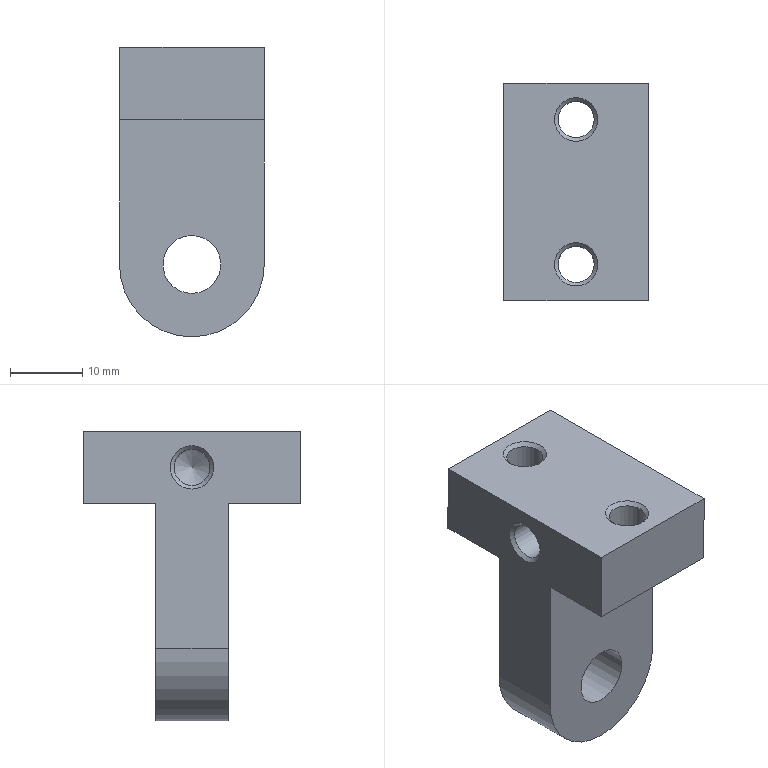Part | STEP file | 冲床-300配套压波_id686_x_t | 1 solid | 20 faces | box 20.046 x 30 x 40.015 mm | volume 10464 mm3 | plane 9 | cone 6 | cylinder 5 | commonest cylinder face diameters 5 x3 8 x1 20 x1
STEP:
#1=CARTESIAN_POINT('',(2189.7,-5.,-434.542));
#2=VERTEX_POINT('',#1);
#3=CARTESIAN_POINT('',(2193.457,-5.,-435.916));
#4=DIRECTION('',(0.,-1.,0.));
#5=DIRECTION('',(-0.9392,0.,0.3435));
#6=AXIS2_PLACEMENT_3D('',#3,#4,#5);
#7=CIRCLE('',#6,4.);
#8=EDGE_CURVE('',#2,#2,#7,.T.);
#9=ORIENTED_EDGE('',*,*,#8,.F.);
#10=EDGE_LOOP('',(#9));
#11=FACE_BOUND('',#10,.T.);
#12=CARTESIAN_POINT('',(2183.488,-5.,-415.901));
#13=VERTEX_POINT('',#12);
#14=CARTESIAN_POINT('',(2203.488,-5.,-415.931));
#15=VERTEX_POINT('',#14);
#16=CARTESIAN_POINT('',(2183.488,-5.,-415.901));
#17=DIRECTION('',(1.,0.,-0.001532));
#18=VECTOR('',#17,1.);
#19=LINE('',#16,#18);
#20=EDGE_CURVE('',#13,#15,#19,.T.);
#21=ORIENTED_EDGE('',*,*,#20,.F.);
#22=CARTESIAN_POINT('',(2183.457,-5.,-435.901));
#23=VERTEX_POINT('',#22);
#24=CARTESIAN_POINT('',(2183.48,-5.,-420.901));
#25=DIRECTION('',(-0.001532,0.,-1.));
#26=VECTOR('',#25,1.);
#27=LINE('',#24,#26);
#28=EDGE_CURVE('',#13,#23,#27,.T.);
#29=ORIENTED_EDGE('',*,*,#28,.T.);
#30=CARTESIAN_POINT('',(2203.457,-5.,-435.931));
#31=VERTEX_POINT('',#30);
#32=CARTESIAN_POINT('',(2193.457,-5.,-435.916));
#33=DIRECTION('',(0.,-1.,0.));
#34=DIRECTION('',(-1.,0.,0.001532));
#35=AXIS2_PLACEMENT_3D('',#32,#33,#34);
#36=CIRCLE('',#35,10.);
#37=EDGE_CURVE('',#23,#31,#36,.T.);
#38=ORIENTED_EDGE('',*,*,#37,.T.);
#39=CARTESIAN_POINT('',(2203.48,-5.,-420.931));
#40=DIRECTION('',(0.001532,0.,1.));
#41=VECTOR('',#40,1.);
#42=LINE('',#39,#41);
#43=EDGE_CURVE('',#31,#15,#42,.T.);
#44=ORIENTED_EDGE('',*,*,#43,.T.);
#45=EDGE_LOOP('',(#21,#29,#38,#44));
#46=FACE_BOUND('',#45,.T.);
#47=CARTESIAN_POINT('',(2183.48,-5.,-420.901));
#48=DIRECTION('',(0.,1.,0.));
#49=DIRECTION('',(1.,0.,-0.001532));
#50=AXIS2_PLACEMENT_3D('',#47,#48,#49);
#51=PLANE('',#50);
#52=ADVANCED_FACE('',(#11,#46),#51,.F.);
#53=CARTESIAN_POINT('',(2203.503,15.,-405.931));
#54=VERTEX_POINT('',#53);
#55=CARTESIAN_POINT('',(2203.503,-15.,-405.931));
#56=VERTEX_POINT('',#55);
#57=CARTESIAN_POINT('',(2203.503,5.,-405.931));
#58=DIRECTION('',(0.,-1.,0.));
#59=VECTOR('',#58,1.);
#60=LINE('',#57,#59);
#61=EDGE_CURVE('',#54,#56,#60,.T.);
#62=ORIENTED_EDGE('',*,*,#61,.T.);
#63=CARTESIAN_POINT('',(2203.488,-15.,-415.931));
#64=VERTEX_POINT('',#63);
#65=CARTESIAN_POINT('',(2203.495,-15.,-410.931));
#66=DIRECTION('',(0.001532,0.,1.));
#67=VECTOR('',#66,1.);
#68=LINE('',#65,#67);
#69=EDGE_CURVE('',#64,#56,#68,.T.);
#70=ORIENTED_EDGE('',*,*,#69,.F.);
#71=CARTESIAN_POINT('',(2203.488,5.,-415.931));
#72=DIRECTION('',(0.,-1.,0.));
#73=VECTOR('',#72,1.);
#74=LINE('',#71,#73);
#75=EDGE_CURVE('',#15,#64,#74,.T.);
#76=ORIENTED_EDGE('',*,*,#75,.F.);
#77=ORIENTED_EDGE('',*,*,#43,.F.);
#78=CARTESIAN_POINT('',(2203.457,5.,-435.931));
#79=VERTEX_POINT('',#78);
#80=CARTESIAN_POINT('',(2203.457,-48.5,-435.931));
#81=DIRECTION('',(0.,1.,0.));
#82=VECTOR('',#81,1.);
#83=LINE('',#80,#82);
#84=EDGE_CURVE('',#31,#79,#83,.T.);
#85=ORIENTED_EDGE('',*,*,#84,.T.);
#86=CARTESIAN_POINT('',(2203.488,5.,-415.931));
#87=VERTEX_POINT('',#86);
#88=CARTESIAN_POINT('',(2203.48,5.,-420.931));
#89=DIRECTION('',(-0.001532,0.,-1.));
#90=VECTOR('',#89,1.);
#91=LINE('',#88,#90);
#92=EDGE_CURVE('',#87,#79,#91,.T.);
#93=ORIENTED_EDGE('',*,*,#92,.F.);
#94=CARTESIAN_POINT('',(2203.488,15.,-415.931));
#95=VERTEX_POINT('',#94);
#96=CARTESIAN_POINT('',(2203.488,-5.,-415.931));
#97=DIRECTION('',(0.,-1.,0.));
#98=VECTOR('',#97,1.);
#99=LINE('',#96,#98);
#100=EDGE_CURVE('',#95,#87,#99,.T.);
#101=ORIENTED_EDGE('',*,*,#100,.F.);
#102=CARTESIAN_POINT('',(2203.495,15.,-410.931));
#103=DIRECTION('',(-0.001532,0.,-1.));
#104=VECTOR('',#103,1.);
#105=LINE('',#102,#104);
#106=EDGE_CURVE('',#54,#95,#105,.T.);
#107=ORIENTED_EDGE('',*,*,#106,.F.);
#108=EDGE_LOOP('',(#62,#70,#76,#77,#85,#93,#101,#107));
#109=FACE_OUTER_BOUND('',#108,.T.);
#110=CARTESIAN_POINT('',(2203.48,5.,-420.931));
#111=DIRECTION('',(1.,0.,-0.001532));
#112=DIRECTION('',(0.,1.,0.));
#113=AXIS2_PLACEMENT_3D('',#110,#111,#112);
#114=PLANE('',#113);
#115=ADVANCED_FACE('',(#109),#114,.T.);
#116=ORIENTED_EDGE('',*,*,#106,.T.);
#117=CARTESIAN_POINT('',(2183.488,15.,-415.901));
#118=VERTEX_POINT('',#117);
#119=CARTESIAN_POINT('',(2183.488,15.,-415.901));
#120=DIRECTION('',(-1.,0.,0.001532));
#121=VECTOR('',#120,1.);
#122=LINE('',#119,#121);
#123=EDGE_CURVE('',#95,#118,#122,.T.);
#124=ORIENTED_EDGE('',*,*,#123,.T.);
#125=CARTESIAN_POINT('',(2183.503,15.,-405.901));
#126=VERTEX_POINT('',#125);
#127=CARTESIAN_POINT('',(2183.495,15.,-410.901));
#128=DIRECTION('',(-0.001532,0.,-1.));
#129=VECTOR('',#128,1.);
#130=LINE('',#127,#129);
#131=EDGE_CURVE('',#126,#118,#130,.T.);
#132=ORIENTED_EDGE('',*,*,#131,.F.);
#133=CARTESIAN_POINT('',(2183.503,15.,-405.901));
#134=DIRECTION('',(-1.,0.,0.001532));
#135=VECTOR('',#134,1.);
#136=LINE('',#133,#135);
#137=EDGE_CURVE('',#54,#126,#136,.T.);
#138=ORIENTED_EDGE('',*,*,#137,.F.);
#139=EDGE_LOOP('',(#116,#124,#132,#138));
#140=FACE_OUTER_BOUND('',#139,.T.);
#141=CARTESIAN_POINT('',(2183.495,15.,-410.901));
#142=DIRECTION('',(0.,-1.,0.));
#143=DIRECTION('',(1.,0.,-0.001532));
#144=AXIS2_PLACEMENT_3D('',#141,#142,#143);
#145=PLANE('',#144);
#146=ADVANCED_FACE('',(#140),#145,.F.);
#147=CARTESIAN_POINT('',(2183.491,0.,-413.901));
#148=VERTEX_POINT('',#147);
#149=CARTESIAN_POINT('',(2183.495,0.,-410.901));
#150=DIRECTION('',(1.,0.,-0.001532));
#151=DIRECTION('',(-0.001532,0.,-1.));
#152=AXIS2_PLACEMENT_3D('',#149,#150,#151);
#153=CIRCLE('',#152,3.);
#154=EDGE_CURVE('',#148,#148,#153,.T.);
#155=ORIENTED_EDGE('',*,*,#154,.T.);
#156=EDGE_LOOP('',(#155));
#157=FACE_BOUND('',#156,.T.);
#158=CARTESIAN_POINT('',(2183.488,5.,-415.901));
#159=VERTEX_POINT('',#158);
#160=CARTESIAN_POINT('',(2183.488,5.,-415.901));
#161=DIRECTION('',(0.,-1.,0.));
#162=VECTOR('',#161,1.);
#163=LINE('',#160,#162);
#164=EDGE_CURVE('',#118,#159,#163,.T.);
#165=ORIENTED_EDGE('',*,*,#164,.T.);
#166=CARTESIAN_POINT('',(2183.457,5.,-435.901));
#167=VERTEX_POINT('',#166);
#168=CARTESIAN_POINT('',(2183.457,5.,-435.901));
#169=DIRECTION('',(0.001532,0.,1.));
#170=VECTOR('',#169,1.);
#171=LINE('',#168,#170);
#172=EDGE_CURVE('',#167,#159,#171,.T.);
#173=ORIENTED_EDGE('',*,*,#172,.F.);
#174=CARTESIAN_POINT('',(2183.457,-48.5,-435.901));
#175=DIRECTION('',(0.,1.,0.));
#176=VECTOR('',#175,1.);
#177=LINE('',#174,#176);
#178=EDGE_CURVE('',#23,#167,#177,.T.);
#179=ORIENTED_EDGE('',*,*,#178,.F.);
#180=ORIENTED_EDGE('',*,*,#28,.F.);
#181=CARTESIAN_POINT('',(2183.488,-15.,-415.901));
#182=VERTEX_POINT('',#181);
#183=CARTESIAN_POINT('',(2183.488,-5.,-415.901));
#184=DIRECTION('',(0.,-1.,0.));
#185=VECTOR('',#184,1.);
#186=LINE('',#183,#185);
#187=EDGE_CURVE('',#13,#182,#186,.T.);
#188=ORIENTED_EDGE('',*,*,#187,.T.);
#189=CARTESIAN_POINT('',(2183.503,-15.,-405.901));
#190=VERTEX_POINT('',#189);
#191=CARTESIAN_POINT('',(2183.495,-15.,-410.901));
#192=DIRECTION('',(0.001532,0.,1.));
#193=VECTOR('',#192,1.);
#194=LINE('',#191,#193);
#195=EDGE_CURVE('',#182,#190,#194,.T.);
#196=ORIENTED_EDGE('',*,*,#195,.T.);
#197=CARTESIAN_POINT('',(2183.503,5.,-405.901));
#198=DIRECTION('',(0.,-1.,0.));
#199=VECTOR('',#198,1.);
#200=LINE('',#197,#199);
#201=EDGE_CURVE('',#126,#190,#200,.T.);
#202=ORIENTED_EDGE('',*,*,#201,.F.);
#203=ORIENTED_EDGE('',*,*,#131,.T.);
#204=EDGE_LOOP('',(#165,#173,#179,#180,#188,#196,#202,#203));
#205=FACE_BOUND('',#204,.T.);
#206=CARTESIAN_POINT('',(2183.48,5.,-420.901));
#207=DIRECTION('',(1.,0.,-0.001532));
#208=DIRECTION('',(0.,1.,0.));
#209=AXIS2_PLACEMENT_3D('',#206,#207,#208);
#210=PLANE('',#209);
#211=ADVANCED_FACE('',(#157,#205),#210,.F.);
#212=CARTESIAN_POINT('',(2190.503,10.,-405.911));
#213=VERTEX_POINT('',#212);
#214=CARTESIAN_POINT('',(2193.503,10.,-405.916));
#215=DIRECTION('',(-0.001532,0.,-1.));
#216=DIRECTION('',(-1.,0.,0.001532));
#217=AXIS2_PLACEMENT_3D('',#214,#215,#216);
#218=CIRCLE('',#217,3.);
#219=EDGE_CURVE('',#213,#213,#218,.T.);
#220=ORIENTED_EDGE('',*,*,#219,.T.);
#221=EDGE_LOOP('',(#220));
#222=FACE_BOUND('',#221,.T.);
#223=CARTESIAN_POINT('',(2190.503,-10.,-405.911));
#224=VERTEX_POINT('',#223);
#225=CARTESIAN_POINT('',(2193.503,-10.,-405.916));
#226=DIRECTION('',(-0.001532,0.,-1.));
#227=DIRECTION('',(-1.,0.,0.001532));
#228=AXIS2_PLACEMENT_3D('',#225,#226,#227);
#229=CIRCLE('',#228,3.);
#230=EDGE_CURVE('',#224,#224,#229,.T.);
#231=ORIENTED_EDGE('',*,*,#230,.T.);
#232=EDGE_LOOP('',(#231));
#233=FACE_BOUND('',#232,.T.);
#234=ORIENTED_EDGE('',*,*,#137,.T.);
#235=ORIENTED_EDGE('',*,*,#201,.T.);
#236=CARTESIAN_POINT('',(2183.503,-15.,-405.901));
#237=DIRECTION('',(1.,0.,-0.001532));
#238=VECTOR('',#237,1.);
#239=LINE('',#236,#238);
#240=EDGE_CURVE('',#190,#56,#239,.T.);
#241=ORIENTED_EDGE('',*,*,#240,.T.);
#242=ORIENTED_EDGE('',*,*,#61,.F.);
#243=EDGE_LOOP('',(#234,#235,#241,#242));
#244=FACE_BOUND('',#243,.T.);
#245=CARTESIAN_POINT('',(2183.503,5.,-405.901));
#246=DIRECTION('',(-0.001532,0.,-1.));
#247=DIRECTION('',(-1.,0.,0.001532));
#248=AXIS2_PLACEMENT_3D('',#245,#246,#247);
#249=PLANE('',#248);
#250=ADVANCED_FACE('',(#222,#233,#244),#249,.F.);
#251=CARTESIAN_POINT('',(2190.488,10.,-415.911));
#252=VERTEX_POINT('',#251);
#253=CARTESIAN_POINT('',(2193.488,10.,-415.916));
#254=DIRECTION('',(0.001532,0.,1.));
#255=DIRECTION('',(-1.,0.,0.001532));
#256=AXIS2_PLACEMENT_3D('',#253,#254,#255);
#257=CIRCLE('',#256,3.);
#258=EDGE_CURVE('',#252,#252,#257,.T.);
#259=ORIENTED_EDGE('',*,*,#258,.T.);
#260=EDGE_LOOP('',(#259));
#261=FACE_BOUND('',#260,.T.);
#262=CARTESIAN_POINT('',(2163.488,5.,-415.87));
#263=DIRECTION('',(1.,0.,-0.001532));
#264=VECTOR('',#263,1.);
#265=LINE('',#262,#264);
#266=EDGE_CURVE('',#159,#87,#265,.T.);
#267=ORIENTED_EDGE('',*,*,#266,.F.);
#268=ORIENTED_EDGE('',*,*,#164,.F.);
#269=ORIENTED_EDGE('',*,*,#123,.F.);
#270=ORIENTED_EDGE('',*,*,#100,.T.);
#271=EDGE_LOOP('',(#267,#268,#269,#270));
#272=FACE_BOUND('',#271,.T.);
#273=CARTESIAN_POINT('',(2183.488,-5.,-415.901));
#274=DIRECTION('',(-0.001532,0.,-1.));
#275=DIRECTION('',(-1.,0.,0.001532));
#276=AXIS2_PLACEMENT_3D('',#273,#274,#275);
#277=PLANE('',#276);
#278=ADVANCED_FACE('',(#261,#272),#277,.T.);
#279=CARTESIAN_POINT('',(2197.214,5.,-437.29));
#280=VERTEX_POINT('',#279);
#281=CARTESIAN_POINT('',(2193.457,5.,-435.916));
#282=DIRECTION('',(0.,1.,0.));
#283=DIRECTION('',(0.9392,0.,-0.3435));
#284=AXIS2_PLACEMENT_3D('',#281,#282,#283);
#285=CIRCLE('',#284,4.);
#286=EDGE_CURVE('',#280,#280,#285,.T.);
#287=ORIENTED_EDGE('',*,*,#286,.F.);
#288=EDGE_LOOP('',(#287));
#289=FACE_BOUND('',#288,.T.);
#290=CARTESIAN_POINT('',(2193.457,5.,-435.916));
#291=DIRECTION('',(0.,1.,0.));
#292=DIRECTION('',(1.,0.,-0.001532));
#293=AXIS2_PLACEMENT_3D('',#290,#291,#292);
#294=CIRCLE('',#293,10.);
#295=EDGE_CURVE('',#79,#167,#294,.T.);
#296=ORIENTED_EDGE('',*,*,#295,.T.);
#297=ORIENTED_EDGE('',*,*,#172,.T.);
#298=ORIENTED_EDGE('',*,*,#266,.T.);
#299=ORIENTED_EDGE('',*,*,#92,.T.);
#300=EDGE_LOOP('',(#296,#297,#298,#299));
#301=FACE_BOUND('',#300,.T.);
#302=CARTESIAN_POINT('',(2163.505,5.,-404.607));
#303=DIRECTION('',(0.,-1.,0.));
#304=DIRECTION('',(1.,0.,-0.001532));
#305=AXIS2_PLACEMENT_3D('',#302,#303,#304);
#306=PLANE('',#305);
#307=ADVANCED_FACE('',(#289,#301),#306,.F.);
#308=ORIENTED_EDGE('',*,*,#37,.F.);
#309=ORIENTED_EDGE('',*,*,#178,.T.);
#310=ORIENTED_EDGE('',*,*,#295,.F.);
#311=ORIENTED_EDGE('',*,*,#84,.F.);
#312=EDGE_LOOP('',(#308,#309,#310,#311));
#313=FACE_OUTER_BOUND('',#312,.T.);
#314=CARTESIAN_POINT('',(2193.457,-48.5,-435.916));
#315=DIRECTION('',(0.,1.,0.));
#316=DIRECTION('',(-1.,0.,0.001532));
#317=AXIS2_PLACEMENT_3D('',#314,#315,#316);
#318=CYLINDRICAL_SURFACE('',#317,10.);
#319=ADVANCED_FACE('',(#313),#318,.T.);
#320=ORIENTED_EDGE('',*,*,#69,.T.);
#321=ORIENTED_EDGE('',*,*,#240,.F.);
#322=ORIENTED_EDGE('',*,*,#195,.F.);
#323=CARTESIAN_POINT('',(2183.488,-15.,-415.901));
#324=DIRECTION('',(1.,0.,-0.001532));
#325=VECTOR('',#324,1.);
#326=LINE('',#323,#325);
#327=EDGE_CURVE('',#182,#64,#326,.T.);
#328=ORIENTED_EDGE('',*,*,#327,.T.);
#329=EDGE_LOOP('',(#320,#321,#322,#328));
#330=FACE_OUTER_BOUND('',#329,.T.);
#331=CARTESIAN_POINT('',(2183.495,-15.,-410.901));
#332=DIRECTION('',(0.,1.,0.));
#333=DIRECTION('',(1.,0.,-0.001532));
#334=AXIS2_PLACEMENT_3D('',#331,#332,#333);
#335=PLANE('',#334);
#336=ADVANCED_FACE('',(#330),#335,.F.);
#337=CARTESIAN_POINT('',(2190.488,-10.,-415.911));
#338=VERTEX_POINT('',#337);
#339=CARTESIAN_POINT('',(2193.488,-10.,-415.916));
#340=DIRECTION('',(0.001532,0.,1.));
#341=DIRECTION('',(-1.,0.,0.001532));
#342=AXIS2_PLACEMENT_3D('',#339,#340,#341);
#343=CIRCLE('',#342,3.);
#344=EDGE_CURVE('',#338,#338,#343,.T.);
#345=ORIENTED_EDGE('',*,*,#344,.T.);
#346=EDGE_LOOP('',(#345));
#347=FACE_BOUND('',#346,.T.);
#348=ORIENTED_EDGE('',*,*,#327,.F.);
#349=ORIENTED_EDGE('',*,*,#187,.F.);
#350=ORIENTED_EDGE('',*,*,#20,.T.);
#351=ORIENTED_EDGE('',*,*,#75,.T.);
#352=EDGE_LOOP('',(#348,#349,#350,#351));
#353=FACE_BOUND('',#352,.T.);
#354=CARTESIAN_POINT('',(2183.488,-5.,-415.901));
#355=DIRECTION('',(-0.001532,0.,-1.));
#356=DIRECTION('',(-1.,0.,0.001532));
#357=AXIS2_PLACEMENT_3D('',#354,#355,#356);
#358=PLANE('',#357);
#359=ADVANCED_FACE('',(#347,#353),#358,.T.);
#360=ORIENTED_EDGE('',*,*,#286,.T.);
#361=EDGE_LOOP('',(#360));
#362=FACE_BOUND('',#361,.T.);
#363=ORIENTED_EDGE('',*,*,#8,.T.);
#364=EDGE_LOOP('',(#363));
#365=FACE_BOUND('',#364,.T.);
#366=CARTESIAN_POINT('',(2193.457,59.,-435.916));
#367=DIRECTION('',(0.,-1.,0.));
#368=DIRECTION('',(1.,0.,-0.001532));
#369=AXIS2_PLACEMENT_3D('',#366,#367,#368);
#370=CYLINDRICAL_SURFACE('',#369,4.);
#371=ADVANCED_FACE('',(#362,#365),#370,.F.);
#372=CARTESIAN_POINT('',(2193.259,0.,-408.416));
#373=VERTEX_POINT('',#372);
#374=CARTESIAN_POINT('',(2193.255,0.,-410.916));
#375=DIRECTION('',(-1.,0.,0.001532));
#376=DIRECTION('',(0.001532,0.,1.));
#377=AXIS2_PLACEMENT_3D('',#374,#375,#376);
#378=CIRCLE('',#377,2.5);
#379=EDGE_CURVE('',#373,#373,#378,.T.);
#380=ORIENTED_EDGE('',*,*,#379,.T.);
#381=EDGE_LOOP('',(#380));
#382=FACE_BOUND('',#381,.T.);
#383=CARTESIAN_POINT('',(2194.757,0.,-410.918));
#384=VERTEX_POINT('',#383);
#385=VERTEX_LOOP('',#384);
#386=FACE_BOUND('',#385,.T.);
#387=CARTESIAN_POINT('',(2193.495,0.,-410.916));
#388=DIRECTION('',(-1.,0.,0.001532));
#389=DIRECTION('',(0.001532,0.,1.));
#390=AXIS2_PLACEMENT_3D('',#387,#388,#389);
#391=CONICAL_SURFACE('',#390,2.1,59.);
#392=ADVANCED_FACE('',(#382,#386),#391,.F.);
#393=CARTESIAN_POINT('',(2183.992,0.,-413.401));
#394=VERTEX_POINT('',#393);
#395=CARTESIAN_POINT('',(2183.995,0.,-410.901));
#396=DIRECTION('',(-1.,0.,0.001532));
#397=DIRECTION('',(-0.001532,0.,-1.));
#398=AXIS2_PLACEMENT_3D('',#395,#396,#397);
#399=CIRCLE('',#398,2.5);
#400=EDGE_CURVE('',#394,#394,#399,.T.);
#401=ORIENTED_EDGE('',*,*,#400,.T.);
#402=EDGE_LOOP('',(#401));
#403=FACE_BOUND('',#402,.T.);
#404=ORIENTED_EDGE('',*,*,#379,.F.);
#405=EDGE_LOOP('',(#404));
#406=FACE_BOUND('',#405,.T.);
#407=CARTESIAN_POINT('',(2183.495,0.,-410.901));
#408=DIRECTION('',(1.,0.,-0.001532));
#409=DIRECTION('',(-0.001532,0.,-1.));
#410=AXIS2_PLACEMENT_3D('',#407,#408,#409);
#411=CYLINDRICAL_SURFACE('',#410,2.5);
#412=ADVANCED_FACE('',(#403,#406),#411,.F.);
#413=CARTESIAN_POINT('',(2190.989,-10.,-415.412));
#414=VERTEX_POINT('',#413);
#415=CARTESIAN_POINT('',(2193.489,-10.,-415.416));
#416=DIRECTION('',(-0.001532,0.,-1.));
#417=DIRECTION('',(-1.,0.,0.001532));
#418=AXIS2_PLACEMENT_3D('',#415,#416,#417);
#419=CIRCLE('',#418,2.5);
#420=EDGE_CURVE('',#414,#414,#419,.T.);
#421=ORIENTED_EDGE('',*,*,#420,.T.);
#422=EDGE_LOOP('',(#421));
#423=FACE_BOUND('',#422,.T.);
#424=CARTESIAN_POINT('',(2191.002,-10.,-406.412));
#425=VERTEX_POINT('',#424);
#426=CARTESIAN_POINT('',(2193.502,-10.,-406.416));
#427=DIRECTION('',(0.001532,0.,1.));
#428=DIRECTION('',(-1.,0.,0.001532));
#429=AXIS2_PLACEMENT_3D('',#426,#427,#428);
#430=CIRCLE('',#429,2.5);
#431=EDGE_CURVE('',#425,#425,#430,.T.);
#432=ORIENTED_EDGE('',*,*,#431,.T.);
#433=EDGE_LOOP('',(#432));
#434=FACE_BOUND('',#433,.T.);
#435=CARTESIAN_POINT('',(2193.503,-10.,-405.916));
#436=DIRECTION('',(-0.001532,0.,-1.));
#437=DIRECTION('',(-1.,0.,0.001532));
#438=AXIS2_PLACEMENT_3D('',#435,#436,#437);
#439=CYLINDRICAL_SURFACE('',#438,2.5);
#440=ADVANCED_FACE('',(#423,#434),#439,.F.);
#441=ORIENTED_EDGE('',*,*,#431,.F.);
#442=EDGE_LOOP('',(#441));
#443=FACE_BOUND('',#442,.T.);
#444=ORIENTED_EDGE('',*,*,#230,.F.);
#445=EDGE_LOOP('',(#444));
#446=FACE_BOUND('',#445,.T.);
#447=CARTESIAN_POINT('',(2193.503,-10.,-405.916));
#448=DIRECTION('',(0.001532,0.,1.));
#449=DIRECTION('',(1.,0.,-0.001532));
#450=AXIS2_PLACEMENT_3D('',#447,#448,#449);
#451=CONICAL_SURFACE('',#450,3.,45.);
#452=ADVANCED_FACE('',(#443,#446),#451,.F.);
#453=ORIENTED_EDGE('',*,*,#344,.F.);
#454=EDGE_LOOP('',(#453));
#455=FACE_BOUND('',#454,.T.);
#456=ORIENTED_EDGE('',*,*,#420,.F.);
#457=EDGE_LOOP('',(#456));
#458=FACE_BOUND('',#457,.T.);
#459=CARTESIAN_POINT('',(2193.489,-10.,-415.416));
#460=DIRECTION('',(-0.001532,0.,-1.));
#461=DIRECTION('',(-1.,0.,0.001532));
#462=AXIS2_PLACEMENT_3D('',#459,#460,#461);
#463=CONICAL_SURFACE('',#462,2.5,45.);
#464=ADVANCED_FACE('',(#455,#458),#463,.F.);
#465=CARTESIAN_POINT('',(2190.989,10.,-415.412));
#466=VERTEX_POINT('',#465);
#467=CARTESIAN_POINT('',(2193.489,10.,-415.416));
#468=DIRECTION('',(-0.001532,0.,-1.));
#469=DIRECTION('',(-1.,0.,0.001532));
#470=AXIS2_PLACEMENT_3D('',#467,#468,#469);
#471=CIRCLE('',#470,2.5);
#472=EDGE_CURVE('',#466,#466,#471,.T.);
#473=ORIENTED_EDGE('',*,*,#472,.T.);
#474=EDGE_LOOP('',(#473));
#475=FACE_BOUND('',#474,.T.);
#476=CARTESIAN_POINT('',(2191.002,10.,-406.412));
#477=VERTEX_POINT('',#476);
#478=CARTESIAN_POINT('',(2193.502,10.,-406.416));
#479=DIRECTION('',(0.001532,0.,1.));
#480=DIRECTION('',(-1.,0.,0.001532));
#481=AXIS2_PLACEMENT_3D('',#478,#479,#480);
#482=CIRCLE('',#481,2.5);
#483=EDGE_CURVE('',#477,#477,#482,.T.);
#484=ORIENTED_EDGE('',*,*,#483,.T.);
#485=EDGE_LOOP('',(#484));
#486=FACE_BOUND('',#485,.T.);
#487=CARTESIAN_POINT('',(2193.503,10.,-405.916));
#488=DIRECTION('',(-0.001532,0.,-1.));
#489=DIRECTION('',(-1.,0.,0.001532));
#490=AXIS2_PLACEMENT_3D('',#487,#488,#489);
#491=CYLINDRICAL_SURFACE('',#490,2.5);
#492=ADVANCED_FACE('',(#475,#486),#491,.F.);
#493=ORIENTED_EDGE('',*,*,#483,.F.);
#494=EDGE_LOOP('',(#493));
#495=FACE_BOUND('',#494,.T.);
#496=ORIENTED_EDGE('',*,*,#219,.F.);
#497=EDGE_LOOP('',(#496));
#498=FACE_BOUND('',#497,.T.);
#499=CARTESIAN_POINT('',(2193.503,10.,-405.916));
#500=DIRECTION('',(0.001532,0.,1.));
#501=DIRECTION('',(1.,0.,-0.001532));
#502=AXIS2_PLACEMENT_3D('',#499,#500,#501);
#503=CONICAL_SURFACE('',#502,3.,45.);
#504=ADVANCED_FACE('',(#495,#498),#503,.F.);
#505=ORIENTED_EDGE('',*,*,#258,.F.);
#506=EDGE_LOOP('',(#505));
#507=FACE_BOUND('',#506,.T.);
#508=ORIENTED_EDGE('',*,*,#472,.F.);
#509=EDGE_LOOP('',(#508));
#510=FACE_BOUND('',#509,.T.);
#511=CARTESIAN_POINT('',(2193.489,10.,-415.416));
#512=DIRECTION('',(-0.001532,0.,-1.));
#513=DIRECTION('',(-1.,0.,0.001532));
#514=AXIS2_PLACEMENT_3D('',#511,#512,#513);
#515=CONICAL_SURFACE('',#514,2.5,45.);
#516=ADVANCED_FACE('',(#507,#510),#515,.F.);
#517=ORIENTED_EDGE('',*,*,#400,.F.);
#518=EDGE_LOOP('',(#517));
#519=FACE_BOUND('',#518,.T.);
#520=ORIENTED_EDGE('',*,*,#154,.F.);
#521=EDGE_LOOP('',(#520));
#522=FACE_BOUND('',#521,.T.);
#523=CARTESIAN_POINT('',(2183.495,0.,-410.901));
#524=DIRECTION('',(-1.,0.,0.001532));
#525=DIRECTION('',(0.001532,0.,1.));
#526=AXIS2_PLACEMENT_3D('',#523,#524,#525);
#527=CONICAL_SURFACE('',#526,3.,45.);
#528=ADVANCED_FACE('',(#519,#522),#527,.F.);
#529=CLOSED_SHELL('',(#52,#115,#146,#211,#250,#278,#307,#319,#336,#359,#371,#392,#412,#440,#452,#464,#492,#504,#516,#528));
#530=MANIFOLD_SOLID_BREP('',#529);
#531=(LENGTH_UNIT()NAMED_UNIT(*)SI_UNIT(.MILLI.,.METRE.));
#532=UNCERTAINTY_MEASURE_WITH_UNIT(LENGTH_MEASURE(0.00002),#531,'','');
#533=(NAMED_UNIT(*)PLANE_ANGLE_UNIT()SI_UNIT($,.RADIAN.));
#534=PLANE_ANGLE_MEASURE_WITH_UNIT(PLANE_ANGLE_MEASURE(0.01745),#533);
#535=DIMENSIONAL_EXPONENTS(0.,0.,0.,0.,0.,0.,0.);
#536=(CONVERSION_BASED_UNIT('DEGREE',#534)NAMED_UNIT(#535)PLANE_ANGLE_UNIT());
#537=(NAMED_UNIT(*)SI_UNIT($,.STERADIAN.)SOLID_ANGLE_UNIT());
#538=(GEOMETRIC_REPRESENTATION_CONTEXT(3)GLOBAL_UNCERTAINTY_ASSIGNED_CONTEXT((#532))GLOBAL_UNIT_ASSIGNED_CONTEXT((#531,#536,#537))REPRESENTATION_CONTEXT('',''));
#539=ADVANCED_BREP_SHAPE_REPRESENTATION('',(#530),#538);